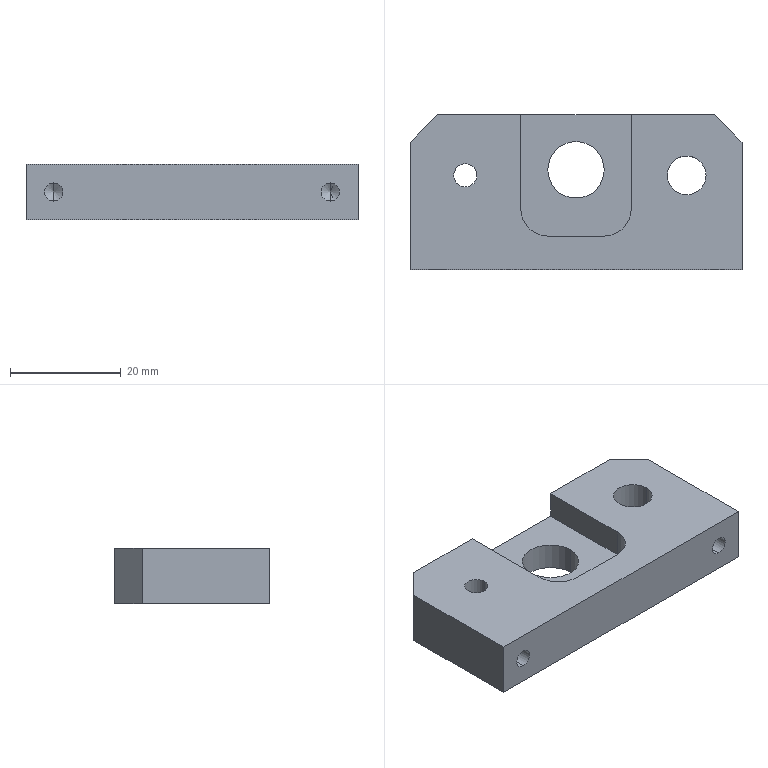Part | STEP file | Mount electronic clip cylinder mounting plate Z-axis | 1 solid | 28 faces | box 60 x 28 x 10 mm | volume 13269 mm3 | cylinder 12 | plane 12 | cone 4 | commonest cylinder face diameters 3.3 x4 4.2 x2 7 x2 10 x2 10.2 x2